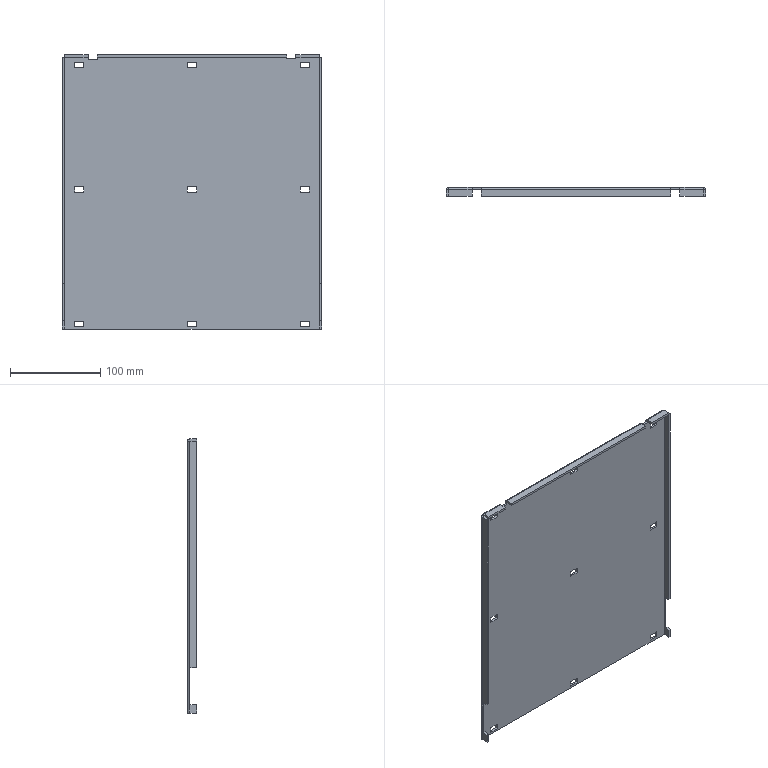Part | NX | features solid 2 | 1 solid | 97 faces | box 287 x 10 x 303.702 mm | volume 229811 mm3 | plane 92 | cylinder 5 | commonest cylinder face diameters 5 x5